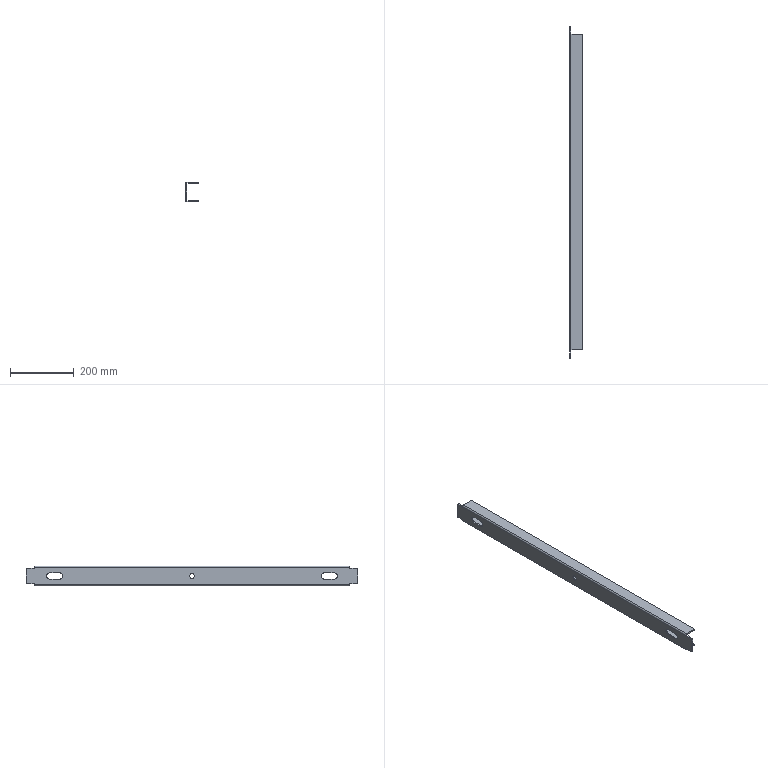Part | 1 solid | 44 faces | box 40 x 1044 x 62 mm | volume 526512 mm3 | plane 30 | cylinder 14 | commonest cylinder face diameters 10 x4 20 x4 0.4 x2 8.4 x2 15 x2
STEP:
#1=CARTESIAN_POINT('',(0.,0.,-7.5));
#2=VERTEX_POINT('',#1);
#3=CARTESIAN_POINT('',(0.,0.,7.5));
#4=VERTEX_POINT('',#3);
#5=CARTESIAN_POINT('',(0.,0.,0.));
#6=DIRECTION('',(-1.,0.,0.));
#7=DIRECTION('',(0.,0.,1.));
#8=AXIS2_PLACEMENT_3D('',#5,#6,#7);
#9=CIRCLE('',#8,7.5);
#10=EDGE_CURVE('',#2,#4,#9,.T.);
#11=ORIENTED_EDGE('',*,*,#10,.T.);
#12=CARTESIAN_POINT('',(4.,0.,7.5));
#13=VERTEX_POINT('',#12);
#14=CARTESIAN_POINT('',(-6.,0.,7.5));
#15=DIRECTION('',(1.,0.,0.));
#16=VECTOR('',#15,1000.);
#17=LINE('',#14,#16);
#18=EDGE_CURVE('',#4,#13,#17,.T.);
#19=ORIENTED_EDGE('',*,*,#18,.T.);
#20=CARTESIAN_POINT('',(4.,0.,-7.5));
#21=VERTEX_POINT('',#20);
#22=CARTESIAN_POINT('',(4.,0.,0.));
#23=DIRECTION('',(1.,0.,0.));
#24=DIRECTION('',(0.,0.,-1.));
#25=AXIS2_PLACEMENT_3D('',#22,#23,#24);
#26=CIRCLE('',#25,7.5);
#27=EDGE_CURVE('',#13,#21,#26,.T.);
#28=ORIENTED_EDGE('',*,*,#27,.T.);
#29=CARTESIAN_POINT('',(-6.,0.,-7.5));
#30=DIRECTION('',(1.,0.,0.));
#31=VECTOR('',#30,1000.);
#32=LINE('',#29,#31);
#33=EDGE_CURVE('',#2,#21,#32,.T.);
#34=ORIENTED_EDGE('',*,*,#33,.F.);
#35=EDGE_LOOP('',(#11,#19,#28,#34));
#36=FACE_OUTER_BOUND('',#35,.T.);
#37=CARTESIAN_POINT('',(-6.,0.,0.));
#38=DIRECTION('',(1.,0.,0.));
#39=DIRECTION('',(0.,0.,-1.));
#40=AXIS2_PLACEMENT_3D('',#37,#38,#39);
#41=CYLINDRICAL_SURFACE('',#40,7.5);
#42=ADVANCED_FACE('',(#36),#41,.F.);
#43=CARTESIAN_POINT('',(4.,-496.,25.));
#44=VERTEX_POINT('',#43);
#45=CARTESIAN_POINT('',(0.,-496.,25.));
#46=VERTEX_POINT('',#45);
#47=CARTESIAN_POINT('',(4.2,-496.,25.));
#48=DIRECTION('',(-1.,0.,0.));
#49=VECTOR('',#48,1000.);
#50=LINE('',#47,#49);
#51=EDGE_CURVE('',#44,#46,#50,.T.);
#52=ORIENTED_EDGE('',*,*,#51,.F.);
#53=CARTESIAN_POINT('',(4.,-496.,26.8));
#54=VERTEX_POINT('',#53);
#55=CARTESIAN_POINT('',(4.,-496.,-31.));
#56=DIRECTION('',(0.,0.,-1.));
#57=VECTOR('',#56,1000.);
#58=LINE('',#55,#57);
#59=EDGE_CURVE('',#54,#44,#58,.T.);
#60=ORIENTED_EDGE('',*,*,#59,.F.);
#61=CARTESIAN_POINT('',(0.,-496.,26.8));
#62=VERTEX_POINT('',#61);
#63=CARTESIAN_POINT('',(4.,-496.,26.8));
#64=DIRECTION('',(-1.,0.,0.));
#65=VECTOR('',#64,1000.);
#66=LINE('',#63,#65);
#67=EDGE_CURVE('',#54,#62,#66,.T.);
#68=ORIENTED_EDGE('',*,*,#67,.T.);
#69=CARTESIAN_POINT('',(0.,-496.,-31.));
#70=DIRECTION('',(0.,0.,-1.));
#71=VECTOR('',#70,1000.);
#72=LINE('',#69,#71);
#73=EDGE_CURVE('',#62,#46,#72,.T.);
#74=ORIENTED_EDGE('',*,*,#73,.T.);
#75=EDGE_LOOP('',(#52,#60,#68,#74));
#76=FACE_OUTER_BOUND('',#75,.T.);
#77=CARTESIAN_POINT('',(4.2,-496.,-27.));
#78=DIRECTION('',(0.,-1.,0.));
#79=DIRECTION('',(0.,0.,-1.));
#80=AXIS2_PLACEMENT_3D('',#77,#78,#79);
#81=PLANE('',#80);
#82=ADVANCED_FACE('',(#76),#81,.T.);
#83=CARTESIAN_POINT('',(4.,496.,-25.));
#84=VERTEX_POINT('',#83);
#85=CARTESIAN_POINT('',(0.,496.,-25.));
#86=VERTEX_POINT('',#85);
#87=CARTESIAN_POINT('',(4.2,496.,-25.));
#88=DIRECTION('',(-1.,0.,0.));
#89=VECTOR('',#88,1000.);
#90=LINE('',#87,#89);
#91=EDGE_CURVE('',#84,#86,#90,.T.);
#92=ORIENTED_EDGE('',*,*,#91,.F.);
#93=CARTESIAN_POINT('',(4.,496.,-26.8));
#94=VERTEX_POINT('',#93);
#95=CARTESIAN_POINT('',(4.,496.,-31.));
#96=DIRECTION('',(0.,0.,-1.));
#97=VECTOR('',#96,1000.);
#98=LINE('',#95,#97);
#99=EDGE_CURVE('',#84,#94,#98,.T.);
#100=ORIENTED_EDGE('',*,*,#99,.T.);
#101=CARTESIAN_POINT('',(0.,496.,-26.8));
#102=VERTEX_POINT('',#101);
#103=CARTESIAN_POINT('',(4.,496.,-26.8));
#104=DIRECTION('',(-1.,0.,0.));
#105=VECTOR('',#104,1000.);
#106=LINE('',#103,#105);
#107=EDGE_CURVE('',#94,#102,#106,.T.);
#108=ORIENTED_EDGE('',*,*,#107,.T.);
#109=CARTESIAN_POINT('',(0.,496.,-31.));
#110=DIRECTION('',(0.,0.,-1.));
#111=VECTOR('',#110,1000.);
#112=LINE('',#109,#111);
#113=EDGE_CURVE('',#86,#102,#112,.T.);
#114=ORIENTED_EDGE('',*,*,#113,.F.);
#115=EDGE_LOOP('',(#92,#100,#108,#114));
#116=FACE_OUTER_BOUND('',#115,.T.);
#117=CARTESIAN_POINT('',(4.2,496.,27.));
#118=DIRECTION('',(0.,1.,0.));
#119=DIRECTION('',(0.,0.,1.));
#120=AXIS2_PLACEMENT_3D('',#117,#118,#119);
#121=PLANE('',#120);
#122=ADVANCED_FACE('',(#116),#121,.T.);
#123=CARTESIAN_POINT('',(0.,496.,26.8));
#124=VERTEX_POINT('',#123);
#125=CARTESIAN_POINT('',(4.,496.,26.8));
#126=VERTEX_POINT('',#125);
#127=CARTESIAN_POINT('',(0.,496.,26.8));
#128=DIRECTION('',(1.,0.,0.));
#129=VECTOR('',#128,1000.);
#130=LINE('',#127,#129);
#131=EDGE_CURVE('',#124,#126,#130,.T.);
#132=ORIENTED_EDGE('',*,*,#131,.F.);
#133=CARTESIAN_POINT('',(4.2,496.,31.));
#134=VERTEX_POINT('',#133);
#135=CARTESIAN_POINT('',(4.2,496.,26.8));
#136=DIRECTION('',(0.,-1.,0.));
#137=DIRECTION('',(0.,0.,1.));
#138=AXIS2_PLACEMENT_3D('',#135,#136,#137);
#139=CIRCLE('',#138,4.2);
#140=EDGE_CURVE('',#134,#124,#139,.T.);
#141=ORIENTED_EDGE('',*,*,#140,.F.);
#142=CARTESIAN_POINT('',(4.2,496.,27.));
#143=VERTEX_POINT('',#142);
#144=CARTESIAN_POINT('',(4.2,496.,27.));
#145=DIRECTION('',(0.,0.,1.));
#146=VECTOR('',#145,1000.);
#147=LINE('',#144,#146);
#148=EDGE_CURVE('',#143,#134,#147,.T.);
#149=ORIENTED_EDGE('',*,*,#148,.F.);
#150=CARTESIAN_POINT('',(4.2,496.,26.8));
#151=DIRECTION('',(0.,-1.,0.));
#152=DIRECTION('',(1.,0.,0.));
#153=AXIS2_PLACEMENT_3D('',#150,#151,#152);
#154=CIRCLE('',#153,0.2);
#155=EDGE_CURVE('',#143,#126,#154,.T.);
#156=ORIENTED_EDGE('',*,*,#155,.T.);
#157=EDGE_LOOP('',(#132,#141,#149,#156));
#158=FACE_OUTER_BOUND('',#157,.T.);
#159=CARTESIAN_POINT('',(0.,496.,26.8));
#160=DIRECTION('',(0.,1.,0.));
#161=DIRECTION('',(0.,0.,1.));
#162=AXIS2_PLACEMENT_3D('',#159,#160,#161);
#163=PLANE('',#162);
#164=ADVANCED_FACE('',(#158),#163,.T.);
#165=CARTESIAN_POINT('',(0.,496.,25.));
#166=VERTEX_POINT('',#165);
#167=CARTESIAN_POINT('',(4.,496.,25.));
#168=VERTEX_POINT('',#167);
#169=CARTESIAN_POINT('',(4.2,496.,25.));
#170=DIRECTION('',(1.,0.,0.));
#171=VECTOR('',#170,1000.);
#172=LINE('',#169,#171);
#173=EDGE_CURVE('',#166,#168,#172,.T.);
#174=ORIENTED_EDGE('',*,*,#173,.F.);
#175=CARTESIAN_POINT('',(0.,496.,-31.));
#176=DIRECTION('',(0.,0.,-1.));
#177=VECTOR('',#176,1000.);
#178=LINE('',#175,#177);
#179=EDGE_CURVE('',#124,#166,#178,.T.);
#180=ORIENTED_EDGE('',*,*,#179,.F.);
#181=ORIENTED_EDGE('',*,*,#131,.T.);
#182=CARTESIAN_POINT('',(4.,496.,-31.));
#183=DIRECTION('',(0.,0.,-1.));
#184=VECTOR('',#183,1000.);
#185=LINE('',#182,#184);
#186=EDGE_CURVE('',#126,#168,#185,.T.);
#187=ORIENTED_EDGE('',*,*,#186,.T.);
#188=EDGE_LOOP('',(#174,#180,#181,#187));
#189=FACE_OUTER_BOUND('',#188,.T.);
#190=CARTESIAN_POINT('',(4.2,496.,27.));
#191=DIRECTION('',(0.,1.,0.));
#192=DIRECTION('',(0.,0.,1.));
#193=AXIS2_PLACEMENT_3D('',#190,#191,#192);
#194=PLANE('',#193);
#195=ADVANCED_FACE('',(#189),#194,.T.);
#196=CARTESIAN_POINT('',(4.2,-496.,31.));
#197=VERTEX_POINT('',#196);
#198=CARTESIAN_POINT('',(4.2,-496.,27.));
#199=VERTEX_POINT('',#198);
#200=CARTESIAN_POINT('',(4.2,-496.,31.));
#201=DIRECTION('',(0.,0.,-1.));
#202=VECTOR('',#201,1000.);
#203=LINE('',#200,#202);
#204=EDGE_CURVE('',#197,#199,#203,.T.);
#205=ORIENTED_EDGE('',*,*,#204,.F.);
#206=CARTESIAN_POINT('',(4.2,-496.,26.8));
#207=DIRECTION('',(0.,-1.,0.));
#208=DIRECTION('',(0.,0.,1.));
#209=AXIS2_PLACEMENT_3D('',#206,#207,#208);
#210=CIRCLE('',#209,4.2);
#211=EDGE_CURVE('',#197,#62,#210,.T.);
#212=ORIENTED_EDGE('',*,*,#211,.T.);
#213=ORIENTED_EDGE('',*,*,#67,.F.);
#214=CARTESIAN_POINT('',(4.2,-496.,26.8));
#215=DIRECTION('',(0.,-1.,0.));
#216=DIRECTION('',(1.,0.,0.));
#217=AXIS2_PLACEMENT_3D('',#214,#215,#216);
#218=CIRCLE('',#217,0.2);
#219=EDGE_CURVE('',#199,#54,#218,.T.);
#220=ORIENTED_EDGE('',*,*,#219,.F.);
#221=EDGE_LOOP('',(#205,#212,#213,#220));
#222=FACE_OUTER_BOUND('',#221,.T.);
#223=CARTESIAN_POINT('',(4.2,-496.,31.));
#224=DIRECTION('',(0.,-1.,0.));
#225=DIRECTION('',(0.,0.,-1.));
#226=AXIS2_PLACEMENT_3D('',#223,#224,#225);
#227=PLANE('',#226);
#228=ADVANCED_FACE('',(#222),#227,.T.);
#229=CARTESIAN_POINT('',(40.,-496.,31.));
#230=VERTEX_POINT('',#229);
#231=CARTESIAN_POINT('',(0.,-496.,31.));
#232=DIRECTION('',(-1.,0.,0.));
#233=VECTOR('',#232,1000.);
#234=LINE('',#231,#233);
#235=EDGE_CURVE('',#230,#197,#234,.T.);
#236=ORIENTED_EDGE('',*,*,#235,.T.);
#237=ORIENTED_EDGE('',*,*,#204,.T.);
#238=CARTESIAN_POINT('',(40.,-496.,27.));
#239=VERTEX_POINT('',#238);
#240=CARTESIAN_POINT('',(0.,-496.,27.));
#241=DIRECTION('',(-1.,0.,0.));
#242=VECTOR('',#241,1000.);
#243=LINE('',#240,#242);
#244=EDGE_CURVE('',#239,#199,#243,.T.);
#245=ORIENTED_EDGE('',*,*,#244,.F.);
#246=CARTESIAN_POINT('',(40.,-496.,27.));
#247=DIRECTION('',(0.,0.,1.));
#248=VECTOR('',#247,1000.);
#249=LINE('',#246,#248);
#250=EDGE_CURVE('',#239,#230,#249,.T.);
#251=ORIENTED_EDGE('',*,*,#250,.T.);
#252=EDGE_LOOP('',(#236,#237,#245,#251));
#253=FACE_OUTER_BOUND('',#252,.T.);
#254=CARTESIAN_POINT('',(4.,-496.,26.8));
#255=DIRECTION('',(0.,-1.,0.));
#256=DIRECTION('',(0.,0.,-1.));
#257=AXIS2_PLACEMENT_3D('',#254,#255,#256);
#258=PLANE('',#257);
#259=ADVANCED_FACE('',(#253),#258,.T.);
#260=CARTESIAN_POINT('',(4.2,496.,-31.));
#261=VERTEX_POINT('',#260);
#262=CARTESIAN_POINT('',(4.2,496.,-27.));
#263=VERTEX_POINT('',#262);
#264=CARTESIAN_POINT('',(4.2,496.,-31.));
#265=DIRECTION('',(0.,0.,1.));
#266=VECTOR('',#265,1000.);
#267=LINE('',#264,#266);
#268=EDGE_CURVE('',#261,#263,#267,.T.);
#269=ORIENTED_EDGE('',*,*,#268,.F.);
#270=CARTESIAN_POINT('',(4.2,496.,-26.8));
#271=DIRECTION('',(0.,-1.,0.));
#272=DIRECTION('',(0.,0.,1.));
#273=AXIS2_PLACEMENT_3D('',#270,#271,#272);
#274=CIRCLE('',#273,4.2);
#275=EDGE_CURVE('',#102,#261,#274,.T.);
#276=ORIENTED_EDGE('',*,*,#275,.F.);
#277=ORIENTED_EDGE('',*,*,#107,.F.);
#278=CARTESIAN_POINT('',(4.2,496.,-26.8));
#279=DIRECTION('',(0.,-1.,0.));
#280=DIRECTION('',(1.,0.,0.));
#281=AXIS2_PLACEMENT_3D('',#278,#279,#280);
#282=CIRCLE('',#281,0.2);
#283=EDGE_CURVE('',#94,#263,#282,.T.);
#284=ORIENTED_EDGE('',*,*,#283,.T.);
#285=EDGE_LOOP('',(#269,#276,#277,#284));
#286=FACE_OUTER_BOUND('',#285,.T.);
#287=CARTESIAN_POINT('',(4.2,496.,-31.));
#288=DIRECTION('',(0.,1.,0.));
#289=DIRECTION('',(0.,0.,1.));
#290=AXIS2_PLACEMENT_3D('',#287,#288,#289);
#291=PLANE('',#290);
#292=ADVANCED_FACE('',(#286),#291,.T.);
#293=CARTESIAN_POINT('',(40.,496.,-31.));
#294=VERTEX_POINT('',#293);
#295=CARTESIAN_POINT('',(0.,496.,-31.));
#296=DIRECTION('',(1.,0.,0.));
#297=VECTOR('',#296,1000.);
#298=LINE('',#295,#297);
#299=EDGE_CURVE('',#261,#294,#298,.T.);
#300=ORIENTED_EDGE('',*,*,#299,.F.);
#301=ORIENTED_EDGE('',*,*,#268,.T.);
#302=CARTESIAN_POINT('',(40.,496.,-27.));
#303=VERTEX_POINT('',#302);
#304=CARTESIAN_POINT('',(0.,496.,-27.));
#305=DIRECTION('',(1.,0.,0.));
#306=VECTOR('',#305,1000.);
#307=LINE('',#304,#306);
#308=EDGE_CURVE('',#263,#303,#307,.T.);
#309=ORIENTED_EDGE('',*,*,#308,.T.);
#310=CARTESIAN_POINT('',(40.,496.,-31.));
#311=DIRECTION('',(0.,0.,1.));
#312=VECTOR('',#311,1000.);
#313=LINE('',#310,#312);
#314=EDGE_CURVE('',#294,#303,#313,.T.);
#315=ORIENTED_EDGE('',*,*,#314,.F.);
#316=EDGE_LOOP('',(#300,#301,#309,#315));
#317=FACE_OUTER_BOUND('',#316,.T.);
#318=CARTESIAN_POINT('',(4.,496.,-26.8));
#319=DIRECTION('',(0.,1.,0.));
#320=DIRECTION('',(0.,0.,1.));
#321=AXIS2_PLACEMENT_3D('',#318,#319,#320);
#322=PLANE('',#321);
#323=ADVANCED_FACE('',(#317),#322,.T.);
#324=CARTESIAN_POINT('',(0.,-496.,-26.8));
#325=VERTEX_POINT('',#324);
#326=CARTESIAN_POINT('',(4.,-496.,-26.8));
#327=VERTEX_POINT('',#326);
#328=CARTESIAN_POINT('',(0.,-496.,-26.8));
#329=DIRECTION('',(1.,0.,0.));
#330=VECTOR('',#329,1000.);
#331=LINE('',#328,#330);
#332=EDGE_CURVE('',#325,#327,#331,.T.);
#333=ORIENTED_EDGE('',*,*,#332,.F.);
#334=CARTESIAN_POINT('',(4.2,-496.,-31.));
#335=VERTEX_POINT('',#334);
#336=CARTESIAN_POINT('',(4.2,-496.,-26.8));
#337=DIRECTION('',(0.,-1.,0.));
#338=DIRECTION('',(0.,0.,1.));
#339=AXIS2_PLACEMENT_3D('',#336,#337,#338);
#340=CIRCLE('',#339,4.2);
#341=EDGE_CURVE('',#325,#335,#340,.T.);
#342=ORIENTED_EDGE('',*,*,#341,.T.);
#343=CARTESIAN_POINT('',(4.2,-496.,-27.));
#344=VERTEX_POINT('',#343);
#345=CARTESIAN_POINT('',(4.2,-496.,-27.));
#346=DIRECTION('',(0.,0.,-1.));
#347=VECTOR('',#346,1000.);
#348=LINE('',#345,#347);
#349=EDGE_CURVE('',#344,#335,#348,.T.);
#350=ORIENTED_EDGE('',*,*,#349,.F.);
#351=CARTESIAN_POINT('',(4.2,-496.,-26.8));
#352=DIRECTION('',(0.,-1.,0.));
#353=DIRECTION('',(1.,0.,0.));
#354=AXIS2_PLACEMENT_3D('',#351,#352,#353);
#355=CIRCLE('',#354,0.2);
#356=EDGE_CURVE('',#327,#344,#355,.T.);
#357=ORIENTED_EDGE('',*,*,#356,.F.);
#358=EDGE_LOOP('',(#333,#342,#350,#357));
#359=FACE_OUTER_BOUND('',#358,.T.);
#360=CARTESIAN_POINT('',(0.,-496.,-26.8));
#361=DIRECTION('',(0.,-1.,0.));
#362=DIRECTION('',(0.,0.,-1.));
#363=AXIS2_PLACEMENT_3D('',#360,#361,#362);
#364=PLANE('',#363);
#365=ADVANCED_FACE('',(#359),#364,.T.);
#366=CARTESIAN_POINT('',(0.,-496.,-25.));
#367=VERTEX_POINT('',#366);
#368=CARTESIAN_POINT('',(4.,-496.,-25.));
#369=VERTEX_POINT('',#368);
#370=CARTESIAN_POINT('',(4.2,-496.,-25.));
#371=DIRECTION('',(1.,0.,0.));
#372=VECTOR('',#371,1000.);
#373=LINE('',#370,#372);
#374=EDGE_CURVE('',#367,#369,#373,.T.);
#375=ORIENTED_EDGE('',*,*,#374,.F.);
#376=CARTESIAN_POINT('',(0.,-496.,-31.));
#377=DIRECTION('',(0.,0.,-1.));
#378=VECTOR('',#377,1000.);
#379=LINE('',#376,#378);
#380=EDGE_CURVE('',#367,#325,#379,.T.);
#381=ORIENTED_EDGE('',*,*,#380,.T.);
#382=ORIENTED_EDGE('',*,*,#332,.T.);
#383=CARTESIAN_POINT('',(4.,-496.,-31.));
#384=DIRECTION('',(0.,0.,-1.));
#385=VECTOR('',#384,1000.);
#386=LINE('',#383,#385);
#387=EDGE_CURVE('',#369,#327,#386,.T.);
#388=ORIENTED_EDGE('',*,*,#387,.F.);
#389=EDGE_LOOP('',(#375,#381,#382,#388));
#390=FACE_OUTER_BOUND('',#389,.T.);
#391=CARTESIAN_POINT('',(4.2,-496.,-27.));
#392=DIRECTION('',(0.,-1.,0.));
#393=DIRECTION('',(0.,0.,-1.));
#394=AXIS2_PLACEMENT_3D('',#391,#392,#393);
#395=PLANE('',#394);
#396=ADVANCED_FACE('',(#390),#395,.T.);
#397=CARTESIAN_POINT('',(40.,-496.,-27.));
#398=VERTEX_POINT('',#397);
#399=CARTESIAN_POINT('',(0.,-496.,-27.));
#400=DIRECTION('',(1.,0.,0.));
#401=VECTOR('',#400,1000.);
#402=LINE('',#399,#401);
#403=EDGE_CURVE('',#344,#398,#402,.T.);
#404=ORIENTED_EDGE('',*,*,#403,.T.);
#405=CARTESIAN_POINT('',(40.,496.,-27.));
#406=DIRECTION('',(0.,-1.,0.));
#407=VECTOR('',#406,1000.);
#408=LINE('',#405,#407);
#409=EDGE_CURVE('',#303,#398,#408,.T.);
#410=ORIENTED_EDGE('',*,*,#409,.F.);
#411=ORIENTED_EDGE('',*,*,#308,.F.);
#412=CARTESIAN_POINT('',(4.2,496.,-27.));
#413=DIRECTION('',(0.,-1.,0.));
#414=VECTOR('',#413,1000.);
#415=LINE('',#412,#414);
#416=EDGE_CURVE('',#263,#344,#415,.T.);
#417=ORIENTED_EDGE('',*,*,#416,.T.);
#418=EDGE_LOOP('',(#404,#410,#411,#417));
#419=FACE_OUTER_BOUND('',#418,.T.);
#420=CARTESIAN_POINT('',(0.,496.,-27.));
#421=DIRECTION('',(0.,0.,-1.));
#422=DIRECTION('',(-1.,0.,0.));
#423=AXIS2_PLACEMENT_3D('',#420,#421,#422);
#424=PLANE('',#423);
#425=ADVANCED_FACE('',(#419),#424,.F.);
#426=CARTESIAN_POINT('',(40.,-496.,-31.));
#427=VERTEX_POINT('',#426);
#428=CARTESIAN_POINT('',(40.,-496.,-31.));
#429=DIRECTION('',(0.,0.,1.));
#430=VECTOR('',#429,1000.);
#431=LINE('',#428,#430);
#432=EDGE_CURVE('',#427,#398,#431,.T.);
#433=ORIENTED_EDGE('',*,*,#432,.F.);
#434=CARTESIAN_POINT('',(40.,496.,-31.));
#435=DIRECTION('',(0.,-1.,0.));
#436=VECTOR('',#435,1000.);
#437=LINE('',#434,#436);
#438=EDGE_CURVE('',#294,#427,#437,.T.);
#439=ORIENTED_EDGE('',*,*,#438,.F.);
#440=ORIENTED_EDGE('',*,*,#314,.T.);
#441=ORIENTED_EDGE('',*,*,#409,.T.);
#442=EDGE_LOOP('',(#433,#439,#440,#441));
#443=FACE_OUTER_BOUND('',#442,.T.);
#444=CARTESIAN_POINT('',(40.,496.,-31.));
#445=DIRECTION('',(1.,0.,0.));
#446=DIRECTION('',(0.,0.,-1.));
#447=AXIS2_PLACEMENT_3D('',#444,#445,#446);
#448=PLANE('',#447);
#449=ADVANCED_FACE('',(#443),#448,.T.);
#450=CARTESIAN_POINT('',(0.,-496.,-31.));
#451=DIRECTION('',(1.,0.,0.));
#452=VECTOR('',#451,1000.);
#453=LINE('',#450,#452);
#454=EDGE_CURVE('',#335,#427,#453,.T.);
#455=ORIENTED_EDGE('',*,*,#454,.F.);
#456=CARTESIAN_POINT('',(4.2,496.,-31.));
#457=DIRECTION('',(0.,-1.,0.));
#458=VECTOR('',#457,1000.);
#459=LINE('',#456,#458);
#460=EDGE_CURVE('',#261,#335,#459,.T.);
#461=ORIENTED_EDGE('',*,*,#460,.F.);
#462=ORIENTED_EDGE('',*,*,#299,.T.);
#463=ORIENTED_EDGE('',*,*,#438,.T.);
#464=EDGE_LOOP('',(#455,#461,#462,#463));
#465=FACE_OUTER_BOUND('',#464,.T.);
#466=CARTESIAN_POINT('',(0.,496.,-31.));
#467=DIRECTION('',(0.,0.,-1.));
#468=DIRECTION('',(-1.,0.,0.));
#469=AXIS2_PLACEMENT_3D('',#466,#467,#468);
#470=PLANE('',#469);
#471=ADVANCED_FACE('',(#465),#470,.T.);
#472=ORIENTED_EDGE('',*,*,#341,.F.);
#473=CARTESIAN_POINT('',(0.,496.,-26.8));
#474=DIRECTION('',(0.,-1.,0.));
#475=VECTOR('',#474,1000.);
#476=LINE('',#473,#475);
#477=EDGE_CURVE('',#102,#325,#476,.T.);
#478=ORIENTED_EDGE('',*,*,#477,.F.);
#479=ORIENTED_EDGE('',*,*,#275,.T.);
#480=ORIENTED_EDGE('',*,*,#460,.T.);
#481=EDGE_LOOP('',(#472,#478,#479,#480));
#482=FACE_OUTER_BOUND('',#481,.T.);
#483=CARTESIAN_POINT('',(4.2,496.,-26.8));
#484=DIRECTION('',(0.,-1.,0.));
#485=DIRECTION('',(0.,0.,-1.));
#486=AXIS2_PLACEMENT_3D('',#483,#484,#485);
#487=CYLINDRICAL_SURFACE('',#486,4.2);
#488=ADVANCED_FACE('',(#482),#487,.T.);
#489=CARTESIAN_POINT('',(0.,417.,-10.));
#490=VERTEX_POINT('',#489);
#491=CARTESIAN_POINT('',(0.,417.,10.));
#492=VERTEX_POINT('',#491);
#493=CARTESIAN_POINT('',(0.,417.,0.));
#494=DIRECTION('',(-1.,0.,0.));
#495=DIRECTION('',(0.,0.,1.));
#496=AXIS2_PLACEMENT_3D('',#493,#494,#495);
#497=CIRCLE('',#496,10.);
#498=EDGE_CURVE('',#490,#492,#497,.T.);
#499=ORIENTED_EDGE('',*,*,#498,.F.);
#500=CARTESIAN_POINT('',(0.,447.,-10.));
#501=VERTEX_POINT('',#500);
#502=CARTESIAN_POINT('',(0.,496.,-10.));
#503=DIRECTION('',(0.,-1.,0.));
#504=VECTOR('',#503,1000.);
#505=LINE('',#502,#504);
#506=EDGE_CURVE('',#501,#490,#505,.T.);
#507=ORIENTED_EDGE('',*,*,#506,.F.);
#508=CARTESIAN_POINT('',(0.,447.,10.));
#509=VERTEX_POINT('',#508);
#510=CARTESIAN_POINT('',(0.,447.,0.));
#511=DIRECTION('',(-1.,0.,0.));
#512=DIRECTION('',(0.,0.,1.));
#513=AXIS2_PLACEMENT_3D('',#510,#511,#512);
#514=CIRCLE('',#513,10.);
#515=EDGE_CURVE('',#509,#501,#514,.T.);
#516=ORIENTED_EDGE('',*,*,#515,.F.);
#517=CARTESIAN_POINT('',(0.,496.,10.));
#518=DIRECTION('',(0.,1.,0.));
#519=VECTOR('',#518,1000.);
#520=LINE('',#517,#519);
#521=EDGE_CURVE('',#492,#509,#520,.T.);
#522=ORIENTED_EDGE('',*,*,#521,.F.);
#523=EDGE_LOOP('',(#499,#507,#516,#522));
#524=FACE_BOUND('',#523,.T.);
#525=ORIENTED_EDGE('',*,*,#10,.F.);
#526=CARTESIAN_POINT('',(0.,0.,0.));
#527=DIRECTION('',(-1.,0.,0.));
#528=DIRECTION('',(0.,0.,1.));
#529=AXIS2_PLACEMENT_3D('',#526,#527,#528);
#530=CIRCLE('',#529,7.5);
#531=EDGE_CURVE('',#4,#2,#530,.T.);
#532=ORIENTED_EDGE('',*,*,#531,.F.);
#533=EDGE_LOOP('',(#525,#532));
#534=FACE_BOUND('',#533,.T.);
#535=CARTESIAN_POINT('',(0.,-417.,10.));
#536=VERTEX_POINT('',#535);
#537=CARTESIAN_POINT('',(0.,-417.,-10.));
#538=VERTEX_POINT('',#537);
#539=CARTESIAN_POINT('',(0.,-417.,0.));
#540=DIRECTION('',(-1.,0.,0.));
#541=DIRECTION('',(0.,0.,1.));
#542=AXIS2_PLACEMENT_3D('',#539,#540,#541);
#543=CIRCLE('',#542,10.);
#544=EDGE_CURVE('',#536,#538,#543,.T.);
#545=ORIENTED_EDGE('',*,*,#544,.F.);
#546=CARTESIAN_POINT('',(0.,-447.,10.));
#547=VERTEX_POINT('',#546);
#548=CARTESIAN_POINT('',(0.,496.,10.));
#549=DIRECTION('',(0.,1.,0.));
#550=VECTOR('',#549,1000.);
#551=LINE('',#548,#550);
#552=EDGE_CURVE('',#547,#536,#551,.T.);
#553=ORIENTED_EDGE('',*,*,#552,.F.);
#554=CARTESIAN_POINT('',(0.,-447.,-10.));
#555=VERTEX_POINT('',#554);
#556=CARTESIAN_POINT('',(0.,-447.,0.));
#557=DIRECTION('',(-1.,0.,0.));
#558=DIRECTION('',(0.,0.,1.));
#559=AXIS2_PLACEMENT_3D('',#556,#557,#558);
#560=CIRCLE('',#559,10.);
#561=EDGE_CURVE('',#555,#547,#560,.T.);
#562=ORIENTED_EDGE('',*,*,#561,.F.);
#563=CARTESIAN_POINT('',(0.,496.,-10.));
#564=DIRECTION('',(0.,-1.,0.));
#565=VECTOR('',#564,1000.);
#566=LINE('',#563,#565);
#567=EDGE_CURVE('',#538,#555,#566,.T.);
#568=ORIENTED_EDGE('',*,*,#567,.F.);
#569=EDGE_LOOP('',(#545,#553,#562,#568));
#570=FACE_BOUND('',#569,.T.);
#571=CARTESIAN_POINT('',(0.,-517.,-25.));
#572=VERTEX_POINT('',#571);
#573=CARTESIAN_POINT('',(0.,-522.,-25.));
#574=DIRECTION('',(0.,1.,0.));
#575=VECTOR('',#574,1000.);
#576=LINE('',#573,#575);
#577=EDGE_CURVE('',#572,#367,#576,.T.);
#578=ORIENTED_EDGE('',*,*,#577,.F.);
#579=CARTESIAN_POINT('',(0.,-522.,-20.));
#580=VERTEX_POINT('',#579);
#581=CARTESIAN_POINT('',(0.,-517.,-20.));
#582=DIRECTION('',(-1.,0.,0.));
#583=DIRECTION('',(0.,0.,1.));
#584=AXIS2_PLACEMENT_3D('',#581,#582,#583);
#585=CIRCLE('',#584,5.);
#586=EDGE_CURVE('',#572,#580,#585,.T.);
#587=ORIENTED_EDGE('',*,*,#586,.T.);
#588=CARTESIAN_POINT('',(0.,-522.,20.));
#589=VERTEX_POINT('',#588);
#590=CARTESIAN_POINT('',(0.,-522.,25.));
#591=DIRECTION('',(0.,0.,-1.));
#592=VECTOR('',#591,1000.);
#593=LINE('',#590,#592);
#594=EDGE_CURVE('',#589,#580,#593,.T.);
#595=ORIENTED_EDGE('',*,*,#594,.F.);
#596=CARTESIAN_POINT('',(0.,-517.,25.));
#597=VERTEX_POINT('',#596);
#598=CARTESIAN_POINT('',(0.,-517.,20.));
#599=DIRECTION('',(-1.,0.,0.));
#600=DIRECTION('',(0.,0.,1.));
#601=AXIS2_PLACEMENT_3D('',#598,#599,#600);
#602=CIRCLE('',#601,5.);
#603=EDGE_CURVE('',#589,#597,#602,.T.);
#604=ORIENTED_EDGE('',*,*,#603,.T.);
#605=CARTESIAN_POINT('',(0.,-522.,25.));
#606=DIRECTION('',(0.,-1.,0.));
#607=VECTOR('',#606,1000.);
#608=LINE('',#605,#607);
#609=EDGE_CURVE('',#46,#597,#608,.T.);
#610=ORIENTED_EDGE('',*,*,#609,.F.);
#611=ORIENTED_EDGE('',*,*,#73,.F.);
#612=CARTESIAN_POINT('',(0.,496.,26.8));
#613=DIRECTION('',(0.,-1.,0.));
#614=VECTOR('',#613,1000.);
#615=LINE('',#612,#614);
#616=EDGE_CURVE('',#124,#62,#615,.T.);
#617=ORIENTED_EDGE('',*,*,#616,.F.);
#618=ORIENTED_EDGE('',*,*,#179,.T.);
#619=CARTESIAN_POINT('',(0.,517.,25.));
#620=VERTEX_POINT('',#619);
#621=CARTESIAN_POINT('',(0.,522.,25.));
#622=DIRECTION('',(0.,-1.,0.));
#623=VECTOR('',#622,1000.);
#624=LINE('',#621,#623);
#625=EDGE_CURVE('',#620,#166,#624,.T.);
#626=ORIENTED_EDGE('',*,*,#625,.F.);
#627=CARTESIAN_POINT('',(0.,522.,20.));
#628=VERTEX_POINT('',#627);
#629=CARTESIAN_POINT('',(0.,517.,20.));
#630=DIRECTION('',(-1.,0.,0.));
#631=DIRECTION('',(0.,0.,1.));
#632=AXIS2_PLACEMENT_3D('',#629,#630,#631);
#633=CIRCLE('',#632,5.);
#634=EDGE_CURVE('',#620,#628,#633,.T.);
#635=ORIENTED_EDGE('',*,*,#634,.T.);
#636=CARTESIAN_POINT('',(0.,522.,-20.));
#637=VERTEX_POINT('',#636);
#638=CARTESIAN_POINT('',(0.,522.,25.));
#639=DIRECTION('',(0.,0.,1.));
#640=VECTOR('',#639,1000.);
#641=LINE('',#638,#640);
#642=EDGE_CURVE('',#637,#628,#641,.T.);
#643=ORIENTED_EDGE('',*,*,#642,.F.);
#644=CARTESIAN_POINT('',(0.,517.,-25.));
#645=VERTEX_POINT('',#644);
#646=CARTESIAN_POINT('',(0.,517.,-20.));
#647=DIRECTION('',(-1.,0.,0.));
#648=DIRECTION('',(0.,0.,1.));
#649=AXIS2_PLACEMENT_3D('',#646,#647,#648);
#650=CIRCLE('',#649,5.);
#651=EDGE_CURVE('',#637,#645,#650,.T.);
#652=ORIENTED_EDGE('',*,*,#651,.T.);
#653=CARTESIAN_POINT('',(0.,522.,-25.));
#654=DIRECTION('',(0.,1.,0.));
#655=VECTOR('',#654,1000.);
#656=LINE('',#653,#655);
#657=EDGE_CURVE('',#86,#645,#656,.T.);
#658=ORIENTED_EDGE('',*,*,#657,.F.);
#659=ORIENTED_EDGE('',*,*,#113,.T.);
#660=ORIENTED_EDGE('',*,*,#477,.T.);
#661=ORIENTED_EDGE('',*,*,#380,.F.);
#662=EDGE_LOOP('',(#578,#587,#595,#604,#610,#611,#617,#618,#626,#635,#643,#652,#658,#659,#660,#661));
#663=FACE_OUTER_BOUND('',#662,.T.);
#664=CARTESIAN_POINT('',(0.,496.,-31.));
#665=DIRECTION('',(-1.,0.,0.));
#666=DIRECTION('',(0.,0.,1.));
#667=AXIS2_PLACEMENT_3D('',#664,#665,#666);
#668=PLANE('',#667);
#669=ADVANCED_FACE('',(#524,#534,#570,#663),#668,.T.);
#670=ORIENTED_EDGE('',*,*,#211,.F.);
#671=CARTESIAN_POINT('',(4.2,496.,31.));
#672=DIRECTION('',(0.,-1.,0.));
#673=VECTOR('',#672,1000.);
#674=LINE('',#671,#673);
#675=EDGE_CURVE('',#134,#197,#674,.T.);
#676=ORIENTED_EDGE('',*,*,#675,.F.);
#677=ORIENTED_EDGE('',*,*,#140,.T.);
#678=ORIENTED_EDGE('',*,*,#616,.T.);
#679=EDGE_LOOP('',(#670,#676,#677,#678));
#680=FACE_OUTER_BOUND('',#679,.T.);
#681=CARTESIAN_POINT('',(4.2,496.,26.8));
#682=DIRECTION('',(0.,-1.,0.));
#683=DIRECTION('',(0.,0.,-1.));
#684=AXIS2_PLACEMENT_3D('',#681,#682,#683);
#685=CYLINDRICAL_SURFACE('',#684,4.2);
#686=ADVANCED_FACE('',(#680),#685,.T.);
#687=ORIENTED_EDGE('',*,*,#235,.F.);
#688=CARTESIAN_POINT('',(40.,496.,31.));
#689=VERTEX_POINT('',#688);
#690=CARTESIAN_POINT('',(40.,496.,31.));
#691=DIRECTION('',(0.,-1.,0.));
#692=VECTOR('',#691,1000.);
#693=LINE('',#690,#692);
#694=EDGE_CURVE('',#689,#230,#693,.T.);
#695=ORIENTED_EDGE('',*,*,#694,.F.);
#696=CARTESIAN_POINT('',(0.,496.,31.));
#697=DIRECTION('',(-1.,0.,0.));
#698=VECTOR('',#697,1000.);
#699=LINE('',#696,#698);
#700=EDGE_CURVE('',#689,#134,#699,.T.);
#701=ORIENTED_EDGE('',*,*,#700,.T.);
#702=ORIENTED_EDGE('',*,*,#675,.T.);
#703=EDGE_LOOP('',(#687,#695,#701,#702));
#704=FACE_OUTER_BOUND('',#703,.T.);
#705=CARTESIAN_POINT('',(0.,496.,31.));
#706=DIRECTION('',(0.,0.,1.));
#707=DIRECTION('',(1.,0.,0.));
#708=AXIS2_PLACEMENT_3D('',#705,#706,#707);
#709=PLANE('',#708);
#710=ADVANCED_FACE('',(#704),#709,.T.);
#711=ORIENTED_EDGE('',*,*,#250,.F.);
#712=CARTESIAN_POINT('',(40.,496.,27.));
#713=VERTEX_POINT('',#712);
#714=CARTESIAN_POINT('',(40.,496.,27.));
#715=DIRECTION('',(0.,-1.,0.));
#716=VECTOR('',#715,1000.);
#717=LINE('',#714,#716);
#718=EDGE_CURVE('',#713,#239,#717,.T.);
#719=ORIENTED_EDGE('',*,*,#718,.F.);
#720=CARTESIAN_POINT('',(40.,496.,27.));
#721=DIRECTION('',(0.,0.,1.));
#722=VECTOR('',#721,1000.);
#723=LINE('',#720,#722);
#724=EDGE_CURVE('',#713,#689,#723,.T.);
#725=ORIENTED_EDGE('',*,*,#724,.T.);
#726=ORIENTED_EDGE('',*,*,#694,.T.);
#727=EDGE_LOOP('',(#711,#719,#725,#726));
#728=FACE_OUTER_BOUND('',#727,.T.);
#729=CARTESIAN_POINT('',(40.,496.,27.));
#730=DIRECTION('',(1.,0.,0.));
#731=DIRECTION('',(0.,0.,-1.));
#732=AXIS2_PLACEMENT_3D('',#729,#730,#731);
#733=PLANE('',#732);
#734=ADVANCED_FACE('',(#728),#733,.T.);
#735=ORIENTED_EDGE('',*,*,#244,.T.);
#736=CARTESIAN_POINT('',(4.2,496.,27.));
#737=DIRECTION('',(0.,-1.,0.));
#738=VECTOR('',#737,1000.);
#739=LINE('',#736,#738);
#740=EDGE_CURVE('',#143,#199,#739,.T.);
#741=ORIENTED_EDGE('',*,*,#740,.F.);
#742=CARTESIAN_POINT('',(0.,496.,27.));
#743=DIRECTION('',(-1.,0.,0.));
#744=VECTOR('',#743,1000.);
#745=LINE('',#742,#744);
#746=EDGE_CURVE('',#713,#143,#745,.T.);
#747=ORIENTED_EDGE('',*,*,#746,.F.);
#748=ORIENTED_EDGE('',*,*,#718,.T.);
#749=EDGE_LOOP('',(#735,#741,#747,#748));
#750=FACE_OUTER_BOUND('',#749,.T.);
#751=CARTESIAN_POINT('',(0.,496.,27.));
#752=DIRECTION('',(0.,0.,1.));
#753=DIRECTION('',(1.,0.,0.));
#754=AXIS2_PLACEMENT_3D('',#751,#752,#753);
#755=PLANE('',#754);
#756=ADVANCED_FACE('',(#750),#755,.F.);
#757=ORIENTED_EDGE('',*,*,#219,.T.);
#758=CARTESIAN_POINT('',(4.,496.,26.8));
#759=DIRECTION('',(0.,-1.,0.));
#760=VECTOR('',#759,1000.);
#761=LINE('',#758,#760);
#762=EDGE_CURVE('',#126,#54,#761,.T.);
#763=ORIENTED_EDGE('',*,*,#762,.F.);
#764=ORIENTED_EDGE('',*,*,#155,.F.);
#765=ORIENTED_EDGE('',*,*,#740,.T.);
#766=EDGE_LOOP('',(#757,#763,#764,#765));
#767=FACE_OUTER_BOUND('',#766,.T.);
#768=CARTESIAN_POINT('',(4.2,496.,26.8));
#769=DIRECTION('',(0.,-1.,0.));
#770=DIRECTION('',(0.,0.,-1.));
#771=AXIS2_PLACEMENT_3D('',#768,#769,#770);
#772=CYLINDRICAL_SURFACE('',#771,0.2);
#773=ADVANCED_FACE('',(#767),#772,.F.);
#774=CARTESIAN_POINT('',(4.,417.,-10.));
#775=VERTEX_POINT('',#774);
#776=CARTESIAN_POINT('',(4.,447.,-10.));
#777=VERTEX_POINT('',#776);
#778=CARTESIAN_POINT('',(4.,417.,-10.));
#779=DIRECTION('',(0.,1.,0.));
#780=VECTOR('',#779,1000.);
#781=LINE('',#778,#780);
#782=EDGE_CURVE('',#775,#777,#781,.T.);
#783=ORIENTED_EDGE('',*,*,#782,.F.);
#784=CARTESIAN_POINT('',(4.,417.,10.));
#785=VERTEX_POINT('',#784);
#786=CARTESIAN_POINT('',(4.,417.,0.));
#787=DIRECTION('',(1.,0.,0.));
#788=DIRECTION('',(0.,0.,-1.));
#789=AXIS2_PLACEMENT_3D('',#786,#787,#788);
#790=CIRCLE('',#789,10.);
#791=EDGE_CURVE('',#785,#775,#790,.T.);
#792=ORIENTED_EDGE('',*,*,#791,.F.);
#793=CARTESIAN_POINT('',(4.,447.,10.));
#794=VERTEX_POINT('',#793);
#795=CARTESIAN_POINT('',(4.,417.,10.));
#796=DIRECTION('',(0.,-1.,0.));
#797=VECTOR('',#796,1000.);
#798=LINE('',#795,#797);
#799=EDGE_CURVE('',#794,#785,#798,.T.);
#800=ORIENTED_EDGE('',*,*,#799,.F.);
#801=CARTESIAN_POINT('',(4.,447.,0.));
#802=DIRECTION('',(1.,0.,0.));
#803=DIRECTION('',(0.,0.,-1.));
#804=AXIS2_PLACEMENT_3D('',#801,#802,#803);
#805=CIRCLE('',#804,10.);
#806=EDGE_CURVE('',#777,#794,#805,.T.);
#807=ORIENTED_EDGE('',*,*,#806,.F.);
#808=EDGE_LOOP('',(#783,#792,#800,#807));
#809=FACE_BOUND('',#808,.T.);
#810=CARTESIAN_POINT('',(4.,0.,0.));
#811=DIRECTION('',(1.,0.,0.));
#812=DIRECTION('',(0.,0.,-1.));
#813=AXIS2_PLACEMENT_3D('',#810,#811,#812);
#814=CIRCLE('',#813,7.5);
#815=EDGE_CURVE('',#21,#13,#814,.T.);
#816=ORIENTED_EDGE('',*,*,#815,.F.);
#817=ORIENTED_EDGE('',*,*,#27,.F.);
#818=EDGE_LOOP('',(#816,#817));
#819=FACE_BOUND('',#818,.T.);
#820=CARTESIAN_POINT('',(4.,-417.,10.));
#821=VERTEX_POINT('',#820);
#822=CARTESIAN_POINT('',(4.,-447.,10.));
#823=VERTEX_POINT('',#822);
#824=CARTESIAN_POINT('',(4.,-417.,10.));
#825=DIRECTION('',(0.,-1.,0.));
#826=VECTOR('',#825,1000.);
#827=LINE('',#824,#826);
#828=EDGE_CURVE('',#821,#823,#827,.T.);
#829=ORIENTED_EDGE('',*,*,#828,.F.);
#830=CARTESIAN_POINT('',(4.,-417.,-10.));
#831=VERTEX_POINT('',#830);
#832=CARTESIAN_POINT('',(4.,-417.,0.));
#833=DIRECTION('',(1.,0.,0.));
#834=DIRECTION('',(0.,0.,1.));
#835=AXIS2_PLACEMENT_3D('',#832,#833,#834);
#836=CIRCLE('',#835,10.);
#837=EDGE_CURVE('',#831,#821,#836,.T.);
#838=ORIENTED_EDGE('',*,*,#837,.F.);
#839=CARTESIAN_POINT('',(4.,-447.,-10.));
#840=VERTEX_POINT('',#839);
#841=CARTESIAN_POINT('',(4.,-417.,-10.));
#842=DIRECTION('',(0.,1.,0.));
#843=VECTOR('',#842,1000.);
#844=LINE('',#841,#843);
#845=EDGE_CURVE('',#840,#831,#844,.T.);
#846=ORIENTED_EDGE('',*,*,#845,.F.);
#847=CARTESIAN_POINT('',(4.,-447.,0.));
#848=DIRECTION('',(1.,0.,0.));
#849=DIRECTION('',(0.,0.,1.));
#850=AXIS2_PLACEMENT_3D('',#847,#848,#849);
#851=CIRCLE('',#850,10.);
#852=EDGE_CURVE('',#823,#840,#851,.T.);
#853=ORIENTED_EDGE('',*,*,#852,.F.);
#854=EDGE_LOOP('',(#829,#838,#846,#853));
#855=FACE_BOUND('',#854,.T.);
#856=CARTESIAN_POINT('',(4.,-522.,20.));
#857=VERTEX_POINT('',#856);
#858=CARTESIAN_POINT('',(4.,-522.,-20.));
#859=VERTEX_POINT('',#858);
#860=CARTESIAN_POINT('',(4.,-522.,25.));
#861=DIRECTION('',(0.,0.,-1.));
#862=VECTOR('',#861,1000.);
#863=LINE('',#860,#862);
#864=EDGE_CURVE('',#857,#859,#863,.T.);
#865=ORIENTED_EDGE('',*,*,#864,.T.);
#866=CARTESIAN_POINT('',(4.,-517.,-25.));
#867=VERTEX_POINT('',#866);
#868=CARTESIAN_POINT('',(4.,-517.,-20.));
#869=DIRECTION('',(1.,0.,0.));
#870=DIRECTION('',(0.,0.,1.));
#871=AXIS2_PLACEMENT_3D('',#868,#869,#870);
#872=CIRCLE('',#871,5.);
#873=EDGE_CURVE('',#859,#867,#872,.T.);
#874=ORIENTED_EDGE('',*,*,#873,.T.);
#875=CARTESIAN_POINT('',(4.,-522.,-25.));
#876=DIRECTION('',(0.,1.,0.));
#877=VECTOR('',#876,1000.);
#878=LINE('',#875,#877);
#879=EDGE_CURVE('',#867,#369,#878,.T.);
#880=ORIENTED_EDGE('',*,*,#879,.T.);
#881=ORIENTED_EDGE('',*,*,#387,.T.);
#882=CARTESIAN_POINT('',(4.,496.,-26.8));
#883=DIRECTION('',(0.,-1.,0.));
#884=VECTOR('',#883,1000.);
#885=LINE('',#882,#884);
#886=EDGE_CURVE('',#94,#327,#885,.T.);
#887=ORIENTED_EDGE('',*,*,#886,.F.);
#888=ORIENTED_EDGE('',*,*,#99,.F.);
#889=CARTESIAN_POINT('',(4.,517.,-25.));
#890=VERTEX_POINT('',#889);
#891=CARTESIAN_POINT('',(4.,522.,-25.));
#892=DIRECTION('',(0.,1.,0.));
#893=VECTOR('',#892,1000.);
#894=LINE('',#891,#893);
#895=EDGE_CURVE('',#84,#890,#894,.T.);
#896=ORIENTED_EDGE('',*,*,#895,.T.);
#897=CARTESIAN_POINT('',(4.,522.,-20.));
#898=VERTEX_POINT('',#897);
#899=CARTESIAN_POINT('',(4.,517.,-20.));
#900=DIRECTION('',(1.,0.,0.));
#901=DIRECTION('',(0.,0.,1.));
#902=AXIS2_PLACEMENT_3D('',#899,#900,#901);
#903=CIRCLE('',#902,5.);
#904=EDGE_CURVE('',#890,#898,#903,.T.);
#905=ORIENTED_EDGE('',*,*,#904,.T.);
#906=CARTESIAN_POINT('',(4.,522.,20.));
#907=VERTEX_POINT('',#906);
#908=CARTESIAN_POINT('',(4.,522.,25.));
#909=DIRECTION('',(0.,0.,1.));
#910=VECTOR('',#909,1000.);
#911=LINE('',#908,#910);
#912=EDGE_CURVE('',#898,#907,#911,.T.);
#913=ORIENTED_EDGE('',*,*,#912,.T.);
#914=CARTESIAN_POINT('',(4.,517.,25.));
#915=VERTEX_POINT('',#914);
#916=CARTESIAN_POINT('',(4.,517.,20.));
#917=DIRECTION('',(1.,0.,0.));
#918=DIRECTION('',(0.,0.,1.));
#919=AXIS2_PLACEMENT_3D('',#916,#917,#918);
#920=CIRCLE('',#919,5.);
#921=EDGE_CURVE('',#907,#915,#920,.T.);
#922=ORIENTED_EDGE('',*,*,#921,.T.);
#923=CARTESIAN_POINT('',(4.,522.,25.));
#924=DIRECTION('',(0.,-1.,0.));
#925=VECTOR('',#924,1000.);
#926=LINE('',#923,#925);
#927=EDGE_CURVE('',#915,#168,#926,.T.);
#928=ORIENTED_EDGE('',*,*,#927,.T.);
#929=ORIENTED_EDGE('',*,*,#186,.F.);
#930=ORIENTED_EDGE('',*,*,#762,.T.);
#931=ORIENTED_EDGE('',*,*,#59,.T.);
#932=CARTESIAN_POINT('',(4.,-517.,25.));
#933=VERTEX_POINT('',#932);
#934=CARTESIAN_POINT('',(4.,-522.,25.));
#935=DIRECTION('',(0.,-1.,0.));
#936=VECTOR('',#935,1000.);
#937=LINE('',#934,#936);
#938=EDGE_CURVE('',#44,#933,#937,.T.);
#939=ORIENTED_EDGE('',*,*,#938,.T.);
#940=CARTESIAN_POINT('',(4.,-517.,20.));
#941=DIRECTION('',(1.,0.,0.));
#942=DIRECTION('',(0.,0.,1.));
#943=AXIS2_PLACEMENT_3D('',#940,#941,#942);
#944=CIRCLE('',#943,5.);
#945=EDGE_CURVE('',#933,#857,#944,.T.);
#946=ORIENTED_EDGE('',*,*,#945,.T.);
#947=EDGE_LOOP('',(#865,#874,#880,#881,#887,#888,#896,#905,#913,#922,#928,#929,#930,#931,#939,#946));
#948=FACE_OUTER_BOUND('',#947,.T.);
#949=CARTESIAN_POINT('',(4.,496.,-31.));
#950=DIRECTION('',(-1.,0.,0.));
#951=DIRECTION('',(0.,0.,1.));
#952=AXIS2_PLACEMENT_3D('',#949,#950,#951);
#953=PLANE('',#952);
#954=ADVANCED_FACE('',(#809,#819,#855,#948),#953,.F.);
#955=ORIENTED_EDGE('',*,*,#356,.T.);
#956=ORIENTED_EDGE('',*,*,#416,.F.);
#957=ORIENTED_EDGE('',*,*,#283,.F.);
#958=ORIENTED_EDGE('',*,*,#886,.T.);
#959=EDGE_LOOP('',(#955,#956,#957,#958));
#960=FACE_OUTER_BOUND('',#959,.T.);
#961=CARTESIAN_POINT('',(4.2,496.,-26.8));
#962=DIRECTION('',(0.,-1.,0.));
#963=DIRECTION('',(0.,0.,-1.));
#964=AXIS2_PLACEMENT_3D('',#961,#962,#963);
#965=CYLINDRICAL_SURFACE('',#964,0.2);
#966=ADVANCED_FACE('',(#960),#965,.F.);
#967=ORIENTED_EDGE('',*,*,#746,.T.);
#968=ORIENTED_EDGE('',*,*,#148,.T.);
#969=ORIENTED_EDGE('',*,*,#700,.F.);
#970=ORIENTED_EDGE('',*,*,#724,.F.);
#971=EDGE_LOOP('',(#967,#968,#969,#970));
#972=FACE_OUTER_BOUND('',#971,.T.);
#973=CARTESIAN_POINT('',(4.2,496.,-26.8));
#974=DIRECTION('',(0.,1.,0.));
#975=DIRECTION('',(1.,0.,0.));
#976=AXIS2_PLACEMENT_3D('',#973,#974,#975);
#977=PLANE('',#976);
#978=ADVANCED_FACE('',(#972),#977,.T.);
#979=ORIENTED_EDGE('',*,*,#403,.F.);
#980=ORIENTED_EDGE('',*,*,#349,.T.);
#981=ORIENTED_EDGE('',*,*,#454,.T.);
#982=ORIENTED_EDGE('',*,*,#432,.T.);
#983=EDGE_LOOP('',(#979,#980,#981,#982));
#984=FACE_OUTER_BOUND('',#983,.T.);
#985=CARTESIAN_POINT('',(4.2,-496.,-26.8));
#986=DIRECTION('',(0.,1.,0.));
#987=DIRECTION('',(1.,0.,0.));
#988=AXIS2_PLACEMENT_3D('',#985,#986,#987);
#989=PLANE('',#988);
#990=ADVANCED_FACE('',(#984),#989,.F.);
#991=ORIENTED_EDGE('',*,*,#657,.T.);
#992=CARTESIAN_POINT('',(0.,517.,-25.));
#993=DIRECTION('',(1.,0.,0.));
#994=VECTOR('',#993,1000.);
#995=LINE('',#992,#994);
#996=EDGE_CURVE('',#645,#890,#995,.T.);
#997=ORIENTED_EDGE('',*,*,#996,.T.);
#998=ORIENTED_EDGE('',*,*,#895,.F.);
#999=ORIENTED_EDGE('',*,*,#91,.T.);
#1000=EDGE_LOOP('',(#991,#997,#998,#999));
#1001=FACE_OUTER_BOUND('',#1000,.T.);
#1002=CARTESIAN_POINT('',(0.,522.,-25.));
#1003=DIRECTION('',(0.,0.,-1.));
#1004=DIRECTION('',(-1.,0.,0.));
#1005=AXIS2_PLACEMENT_3D('',#1002,#1003,#1004);
#1006=PLANE('',#1005);
#1007=ADVANCED_FACE('',(#1001),#1006,.T.);
#1008=ORIENTED_EDGE('',*,*,#927,.F.);
#1009=CARTESIAN_POINT('',(0.,517.,25.));
#1010=DIRECTION('',(-1.,0.,0.));
#1011=VECTOR('',#1010,1000.);
#1012=LINE('',#1009,#1011);
#1013=EDGE_CURVE('',#915,#620,#1012,.T.);
#1014=ORIENTED_EDGE('',*,*,#1013,.T.);
#1015=ORIENTED_EDGE('',*,*,#625,.T.);
#1016=ORIENTED_EDGE('',*,*,#173,.T.);
#1017=EDGE_LOOP('',(#1008,#1014,#1015,#1016));
#1018=FACE_OUTER_BOUND('',#1017,.T.);
#1019=CARTESIAN_POINT('',(0.,522.,25.));
#1020=DIRECTION('',(0.,0.,1.));
#1021=DIRECTION('',(1.,0.,0.));
#1022=AXIS2_PLACEMENT_3D('',#1019,#1020,#1021);
#1023=PLANE('',#1022);
#1024=ADVANCED_FACE('',(#1018),#1023,.T.);
#1025=ORIENTED_EDGE('',*,*,#642,.T.);
#1026=CARTESIAN_POINT('',(0.,522.,20.));
#1027=DIRECTION('',(1.,0.,0.));
#1028=VECTOR('',#1027,1000.);
#1029=LINE('',#1026,#1028);
#1030=EDGE_CURVE('',#628,#907,#1029,.T.);
#1031=ORIENTED_EDGE('',*,*,#1030,.T.);
#1032=ORIENTED_EDGE('',*,*,#912,.F.);
#1033=CARTESIAN_POINT('',(0.,522.,-20.));
#1034=DIRECTION('',(-1.,0.,0.));
#1035=VECTOR('',#1034,1000.);
#1036=LINE('',#1033,#1035);
#1037=EDGE_CURVE('',#898,#637,#1036,.T.);
#1038=ORIENTED_EDGE('',*,*,#1037,.T.);
#1039=EDGE_LOOP('',(#1025,#1031,#1032,#1038));
#1040=FACE_OUTER_BOUND('',#1039,.T.);
#1041=CARTESIAN_POINT('',(0.,522.,25.));
#1042=DIRECTION('',(0.,1.,0.));
#1043=DIRECTION('',(0.,0.,1.));
#1044=AXIS2_PLACEMENT_3D('',#1041,#1042,#1043);
#1045=PLANE('',#1044);
#1046=ADVANCED_FACE('',(#1040),#1045,.T.);
#1047=ORIENTED_EDGE('',*,*,#609,.T.);
#1048=CARTESIAN_POINT('',(0.,-517.,25.));
#1049=DIRECTION('',(1.,0.,0.));
#1050=VECTOR('',#1049,1000.);
#1051=LINE('',#1048,#1050);
#1052=EDGE_CURVE('',#597,#933,#1051,.T.);
#1053=ORIENTED_EDGE('',*,*,#1052,.T.);
#1054=ORIENTED_EDGE('',*,*,#938,.F.);
#1055=ORIENTED_EDGE('',*,*,#51,.T.);
#1056=EDGE_LOOP('',(#1047,#1053,#1054,#1055));
#1057=FACE_OUTER_BOUND('',#1056,.T.);
#1058=CARTESIAN_POINT('',(0.,-522.,25.));
#1059=DIRECTION('',(0.,0.,1.));
#1060=DIRECTION('',(1.,0.,0.));
#1061=AXIS2_PLACEMENT_3D('',#1058,#1059,#1060);
#1062=PLANE('',#1061);
#1063=ADVANCED_FACE('',(#1057),#1062,.T.);
#1064=ORIENTED_EDGE('',*,*,#879,.F.);
#1065=CARTESIAN_POINT('',(0.,-517.,-25.));
#1066=DIRECTION('',(-1.,0.,0.));
#1067=VECTOR('',#1066,1000.);
#1068=LINE('',#1065,#1067);
#1069=EDGE_CURVE('',#867,#572,#1068,.T.);
#1070=ORIENTED_EDGE('',*,*,#1069,.T.);
#1071=ORIENTED_EDGE('',*,*,#577,.T.);
#1072=ORIENTED_EDGE('',*,*,#374,.T.);
#1073=EDGE_LOOP('',(#1064,#1070,#1071,#1072));
#1074=FACE_OUTER_BOUND('',#1073,.T.);
#1075=CARTESIAN_POINT('',(0.,-522.,-25.));
#1076=DIRECTION('',(0.,0.,-1.));
#1077=DIRECTION('',(-1.,0.,0.));
#1078=AXIS2_PLACEMENT_3D('',#1075,#1076,#1077);
#1079=PLANE('',#1078);
#1080=ADVANCED_FACE('',(#1074),#1079,.T.);
#1081=ORIENTED_EDGE('',*,*,#594,.T.);
#1082=CARTESIAN_POINT('',(0.,-522.,-20.));
#1083=DIRECTION('',(1.,0.,0.));
#1084=VECTOR('',#1083,1000.);
#1085=LINE('',#1082,#1084);
#1086=EDGE_CURVE('',#580,#859,#1085,.T.);
#1087=ORIENTED_EDGE('',*,*,#1086,.T.);
#1088=ORIENTED_EDGE('',*,*,#864,.F.);
#1089=CARTESIAN_POINT('',(0.,-522.,20.));
#1090=DIRECTION('',(-1.,0.,0.));
#1091=VECTOR('',#1090,1000.);
#1092=LINE('',#1089,#1091);
#1093=EDGE_CURVE('',#857,#589,#1092,.T.);
#1094=ORIENTED_EDGE('',*,*,#1093,.T.);
#1095=EDGE_LOOP('',(#1081,#1087,#1088,#1094));
#1096=FACE_OUTER_BOUND('',#1095,.T.);
#1097=CARTESIAN_POINT('',(0.,-522.,25.));
#1098=DIRECTION('',(0.,-1.,0.));
#1099=DIRECTION('',(0.,0.,-1.));
#1100=AXIS2_PLACEMENT_3D('',#1097,#1098,#1099);
#1101=PLANE('',#1100);
#1102=ADVANCED_FACE('',(#1096),#1101,.T.);
#1103=ORIENTED_EDGE('',*,*,#586,.F.);
#1104=ORIENTED_EDGE('',*,*,#1069,.F.);
#1105=ORIENTED_EDGE('',*,*,#873,.F.);
#1106=ORIENTED_EDGE('',*,*,#1086,.F.);
#1107=EDGE_LOOP('',(#1103,#1104,#1105,#1106));
#1108=FACE_OUTER_BOUND('',#1107,.T.);
#1109=CARTESIAN_POINT('',(0.,-517.,-20.));
#1110=DIRECTION('',(1.,0.,0.));
#1111=DIRECTION('',(0.,0.,-1.));
#1112=AXIS2_PLACEMENT_3D('',#1109,#1110,#1111);
#1113=CYLINDRICAL_SURFACE('',#1112,5.);
#1114=ADVANCED_FACE('',(#1108),#1113,.T.);
#1115=ORIENTED_EDGE('',*,*,#603,.F.);
#1116=ORIENTED_EDGE('',*,*,#1093,.F.);
#1117=ORIENTED_EDGE('',*,*,#945,.F.);
#1118=ORIENTED_EDGE('',*,*,#1052,.F.);
#1119=EDGE_LOOP('',(#1115,#1116,#1117,#1118));
#1120=FACE_OUTER_BOUND('',#1119,.T.);
#1121=CARTESIAN_POINT('',(0.,-517.,20.));
#1122=DIRECTION('',(1.,0.,0.));
#1123=DIRECTION('',(0.,0.,-1.));
#1124=AXIS2_PLACEMENT_3D('',#1121,#1122,#1123);
#1125=CYLINDRICAL_SURFACE('',#1124,5.);
#1126=ADVANCED_FACE('',(#1120),#1125,.T.);
#1127=ORIENTED_EDGE('',*,*,#634,.F.);
#1128=ORIENTED_EDGE('',*,*,#1013,.F.);
#1129=ORIENTED_EDGE('',*,*,#921,.F.);
#1130=ORIENTED_EDGE('',*,*,#1030,.F.);
#1131=EDGE_LOOP('',(#1127,#1128,#1129,#1130));
#1132=FACE_OUTER_BOUND('',#1131,.T.);
#1133=CARTESIAN_POINT('',(0.,517.,20.));
#1134=DIRECTION('',(1.,0.,0.));
#1135=DIRECTION('',(0.,0.,-1.));
#1136=AXIS2_PLACEMENT_3D('',#1133,#1134,#1135);
#1137=CYLINDRICAL_SURFACE('',#1136,5.);
#1138=ADVANCED_FACE('',(#1132),#1137,.T.);
#1139=ORIENTED_EDGE('',*,*,#651,.F.);
#1140=ORIENTED_EDGE('',*,*,#1037,.F.);
#1141=ORIENTED_EDGE('',*,*,#904,.F.);
#1142=ORIENTED_EDGE('',*,*,#996,.F.);
#1143=EDGE_LOOP('',(#1139,#1140,#1141,#1142));
#1144=FACE_OUTER_BOUND('',#1143,.T.);
#1145=CARTESIAN_POINT('',(0.,517.,-20.));
#1146=DIRECTION('',(1.,0.,0.));
#1147=DIRECTION('',(0.,0.,-1.));
#1148=AXIS2_PLACEMENT_3D('',#1145,#1146,#1147);
#1149=CYLINDRICAL_SURFACE('',#1148,5.);
#1150=ADVANCED_FACE('',(#1144),#1149,.T.);
#1151=ORIENTED_EDGE('',*,*,#544,.T.);
#1152=CARTESIAN_POINT('',(-6.,-417.,-10.));
#1153=DIRECTION('',(1.,0.,0.));
#1154=VECTOR('',#1153,1000.);
#1155=LINE('',#1152,#1154);
#1156=EDGE_CURVE('',#538,#831,#1155,.T.);
#1157=ORIENTED_EDGE('',*,*,#1156,.T.);
#1158=ORIENTED_EDGE('',*,*,#837,.T.);
#1159=CARTESIAN_POINT('',(-6.,-417.,10.));
#1160=DIRECTION('',(1.,0.,0.));
#1161=VECTOR('',#1160,1000.);
#1162=LINE('',#1159,#1161);
#1163=EDGE_CURVE('',#536,#821,#1162,.T.);
#1164=ORIENTED_EDGE('',*,*,#1163,.F.);
#1165=EDGE_LOOP('',(#1151,#1157,#1158,#1164));
#1166=FACE_OUTER_BOUND('',#1165,.T.);
#1167=CARTESIAN_POINT('',(-6.,-417.,0.));
#1168=DIRECTION('',(1.,0.,0.));
#1169=DIRECTION('',(0.,0.,-1.));
#1170=AXIS2_PLACEMENT_3D('',#1167,#1168,#1169);
#1171=CYLINDRICAL_SURFACE('',#1170,10.);
#1172=ADVANCED_FACE('',(#1166),#1171,.F.);
#1173=ORIENTED_EDGE('',*,*,#567,.T.);
#1174=CARTESIAN_POINT('',(-6.,-447.,-10.));
#1175=DIRECTION('',(1.,0.,0.));
#1176=VECTOR('',#1175,1000.);
#1177=LINE('',#1174,#1176);
#1178=EDGE_CURVE('',#555,#840,#1177,.T.);
#1179=ORIENTED_EDGE('',*,*,#1178,.T.);
#1180=ORIENTED_EDGE('',*,*,#845,.T.);
#1181=ORIENTED_EDGE('',*,*,#1156,.F.);
#1182=EDGE_LOOP('',(#1173,#1179,#1180,#1181));
#1183=FACE_OUTER_BOUND('',#1182,.T.);
#1184=CARTESIAN_POINT('',(-6.,-417.,-10.));
#1185=DIRECTION('',(0.,0.,-1.));
#1186=DIRECTION('',(-1.,0.,0.));
#1187=AXIS2_PLACEMENT_3D('',#1184,#1185,#1186);
#1188=PLANE('',#1187);
#1189=ADVANCED_FACE('',(#1183),#1188,.F.);
#1190=ORIENTED_EDGE('',*,*,#561,.T.);
#1191=CARTESIAN_POINT('',(-6.,-447.,10.));
#1192=DIRECTION('',(1.,0.,0.));
#1193=VECTOR('',#1192,1000.);
#1194=LINE('',#1191,#1193);
#1195=EDGE_CURVE('',#547,#823,#1194,.T.);
#1196=ORIENTED_EDGE('',*,*,#1195,.T.);
#1197=ORIENTED_EDGE('',*,*,#852,.T.);
#1198=ORIENTED_EDGE('',*,*,#1178,.F.);
#1199=EDGE_LOOP('',(#1190,#1196,#1197,#1198));
#1200=FACE_OUTER_BOUND('',#1199,.T.);
#1201=CARTESIAN_POINT('',(-6.,-447.,0.));
#1202=DIRECTION('',(1.,0.,0.));
#1203=DIRECTION('',(0.,0.,-1.));
#1204=AXIS2_PLACEMENT_3D('',#1201,#1202,#1203);
#1205=CYLINDRICAL_SURFACE('',#1204,10.);
#1206=ADVANCED_FACE('',(#1200),#1205,.F.);
#1207=ORIENTED_EDGE('',*,*,#552,.T.);
#1208=ORIENTED_EDGE('',*,*,#1163,.T.);
#1209=ORIENTED_EDGE('',*,*,#828,.T.);
#1210=ORIENTED_EDGE('',*,*,#1195,.F.);
#1211=EDGE_LOOP('',(#1207,#1208,#1209,#1210));
#1212=FACE_OUTER_BOUND('',#1211,.T.);
#1213=CARTESIAN_POINT('',(-6.,-417.,10.));
#1214=DIRECTION('',(0.,0.,1.));
#1215=DIRECTION('',(1.,0.,0.));
#1216=AXIS2_PLACEMENT_3D('',#1213,#1214,#1215);
#1217=PLANE('',#1216);
#1218=ADVANCED_FACE('',(#1212),#1217,.F.);
#1219=ORIENTED_EDGE('',*,*,#18,.F.);
#1220=ORIENTED_EDGE('',*,*,#531,.T.);
#1221=ORIENTED_EDGE('',*,*,#33,.T.);
#1222=ORIENTED_EDGE('',*,*,#815,.T.);
#1223=EDGE_LOOP('',(#1219,#1220,#1221,#1222));
#1224=FACE_OUTER_BOUND('',#1223,.T.);
#1225=CARTESIAN_POINT('',(-6.,0.,0.));
#1226=DIRECTION('',(1.,0.,0.));
#1227=DIRECTION('',(0.,0.,-1.));
#1228=AXIS2_PLACEMENT_3D('',#1225,#1226,#1227);
#1229=CYLINDRICAL_SURFACE('',#1228,7.5);
#1230=ADVANCED_FACE('',(#1224),#1229,.F.);
#1231=ORIENTED_EDGE('',*,*,#498,.T.);
#1232=CARTESIAN_POINT('',(-6.,417.,10.));
#1233=DIRECTION('',(1.,0.,0.));
#1234=VECTOR('',#1233,1000.);
#1235=LINE('',#1232,#1234);
#1236=EDGE_CURVE('',#492,#785,#1235,.T.);
#1237=ORIENTED_EDGE('',*,*,#1236,.T.);
#1238=ORIENTED_EDGE('',*,*,#791,.T.);
#1239=CARTESIAN_POINT('',(-6.,417.,-10.));
#1240=DIRECTION('',(1.,0.,0.));
#1241=VECTOR('',#1240,1000.);
#1242=LINE('',#1239,#1241);
#1243=EDGE_CURVE('',#490,#775,#1242,.T.);
#1244=ORIENTED_EDGE('',*,*,#1243,.F.);
#1245=EDGE_LOOP('',(#1231,#1237,#1238,#1244));
#1246=FACE_OUTER_BOUND('',#1245,.T.);
#1247=CARTESIAN_POINT('',(-6.,417.,0.));
#1248=DIRECTION('',(1.,0.,0.));
#1249=DIRECTION('',(0.,0.,-1.));
#1250=AXIS2_PLACEMENT_3D('',#1247,#1248,#1249);
#1251=CYLINDRICAL_SURFACE('',#1250,10.);
#1252=ADVANCED_FACE('',(#1246),#1251,.F.);
#1253=ORIENTED_EDGE('',*,*,#521,.T.);
#1254=CARTESIAN_POINT('',(-6.,447.,10.));
#1255=DIRECTION('',(1.,0.,0.));
#1256=VECTOR('',#1255,1000.);
#1257=LINE('',#1254,#1256);
#1258=EDGE_CURVE('',#509,#794,#1257,.T.);
#1259=ORIENTED_EDGE('',*,*,#1258,.T.);
#1260=ORIENTED_EDGE('',*,*,#799,.T.);
#1261=ORIENTED_EDGE('',*,*,#1236,.F.);
#1262=EDGE_LOOP('',(#1253,#1259,#1260,#1261));
#1263=FACE_OUTER_BOUND('',#1262,.T.);
#1264=CARTESIAN_POINT('',(-6.,417.,10.));
#1265=DIRECTION('',(0.,0.,1.));
#1266=DIRECTION('',(1.,0.,0.));
#1267=AXIS2_PLACEMENT_3D('',#1264,#1265,#1266);
#1268=PLANE('',#1267);
#1269=ADVANCED_FACE('',(#1263),#1268,.F.);
#1270=ORIENTED_EDGE('',*,*,#515,.T.);
#1271=CARTESIAN_POINT('',(-6.,447.,-10.));
#1272=DIRECTION('',(1.,0.,0.));
#1273=VECTOR('',#1272,1000.);
#1274=LINE('',#1271,#1273);
#1275=EDGE_CURVE('',#501,#777,#1274,.T.);
#1276=ORIENTED_EDGE('',*,*,#1275,.T.);
#1277=ORIENTED_EDGE('',*,*,#806,.T.);
#1278=ORIENTED_EDGE('',*,*,#1258,.F.);
#1279=EDGE_LOOP('',(#1270,#1276,#1277,#1278));
#1280=FACE_OUTER_BOUND('',#1279,.T.);
#1281=CARTESIAN_POINT('',(-6.,447.,0.));
#1282=DIRECTION('',(1.,0.,0.));
#1283=DIRECTION('',(0.,0.,-1.));
#1284=AXIS2_PLACEMENT_3D('',#1281,#1282,#1283);
#1285=CYLINDRICAL_SURFACE('',#1284,10.);
#1286=ADVANCED_FACE('',(#1280),#1285,.F.);
#1287=ORIENTED_EDGE('',*,*,#506,.T.);
#1288=ORIENTED_EDGE('',*,*,#1243,.T.);
#1289=ORIENTED_EDGE('',*,*,#782,.T.);
#1290=ORIENTED_EDGE('',*,*,#1275,.F.);
#1291=EDGE_LOOP('',(#1287,#1288,#1289,#1290));
#1292=FACE_OUTER_BOUND('',#1291,.T.);
#1293=CARTESIAN_POINT('',(-6.,417.,-10.));
#1294=DIRECTION('',(0.,0.,-1.));
#1295=DIRECTION('',(-1.,0.,0.));
#1296=AXIS2_PLACEMENT_3D('',#1293,#1294,#1295);
#1297=PLANE('',#1296);
#1298=ADVANCED_FACE('',(#1292),#1297,.F.);
#1299=CLOSED_SHELL('',(#42,#82,#122,#164,#195,#228,#259,#292,#323,#365,#396,#425,#449,#471,#488,#669,#686,#710,#734,#756,#773,#954,#966,#978,#990,#1007,#1024,#1046,#1063,#1080,#1102,#1114,#1126,#1138,#1150,#1172,#1189,#1206,#1218,#1230,#1252,#1269,#1286,#1298));
#1300=MANIFOLD_SOLID_BREP('',#1299);
#1301=CARTESIAN_POINT('',(0.,0.,0.));
#1302=DIRECTION('',(0.,0.,1.));
#1303=DIRECTION('',(1.,0.,0.));
#1304=AXIS2_PLACEMENT_3D('',#1301,#1302,#1303);
#1305=(LENGTH_UNIT()NAMED_UNIT(*)SI_UNIT(.MILLI.,.METRE.));
#1306=UNCERTAINTY_MEASURE_WITH_UNIT(LENGTH_MEASURE(0.00001),#1305,'','');
#1307=(NAMED_UNIT(*)PLANE_ANGLE_UNIT()SI_UNIT($,.RADIAN.));
#1308=(NAMED_UNIT(*)SI_UNIT($,.STERADIAN.)SOLID_ANGLE_UNIT());
#1309=(GEOMETRIC_REPRESENTATION_CONTEXT(3)GLOBAL_UNCERTAINTY_ASSIGNED_CONTEXT((#1306))GLOBAL_UNIT_ASSIGNED_CONTEXT((#1305,#1307,#1308))REPRESENTATION_CONTEXT('',''));
#1310=ADVANCED_BREP_SHAPE_REPRESENTATION('',(#1300,#1304),#1309);